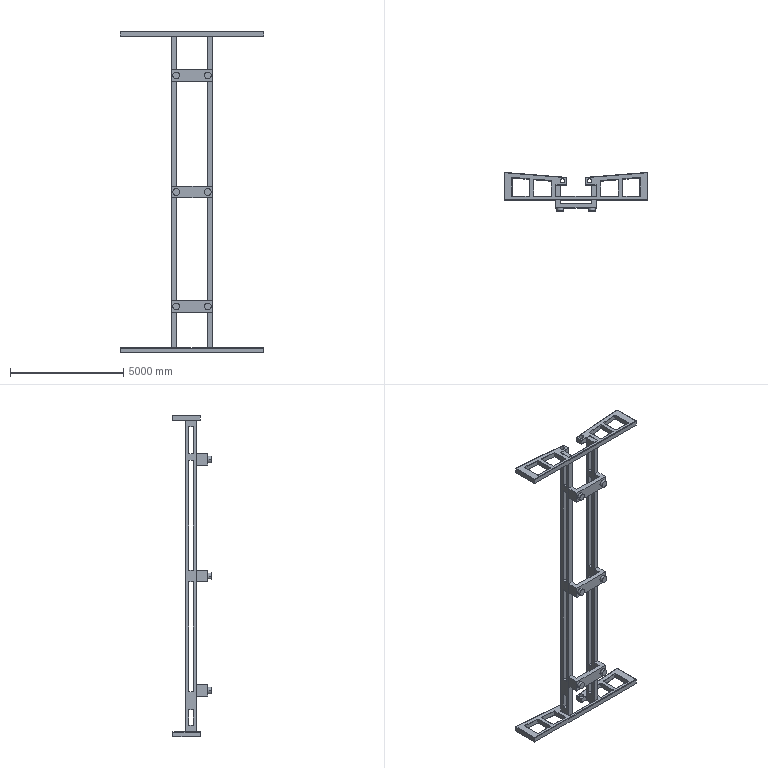Part | SolidWorks | 7 solids | 414 faces | box 6350 x 1686 x 14220 mm | volume 4157610963 mm3 | cylinder 174 | plane 144 | torus 80 | sphere 16 | commonest cylinder face diameters 20 x96 30 x58 300 x12 200 x8